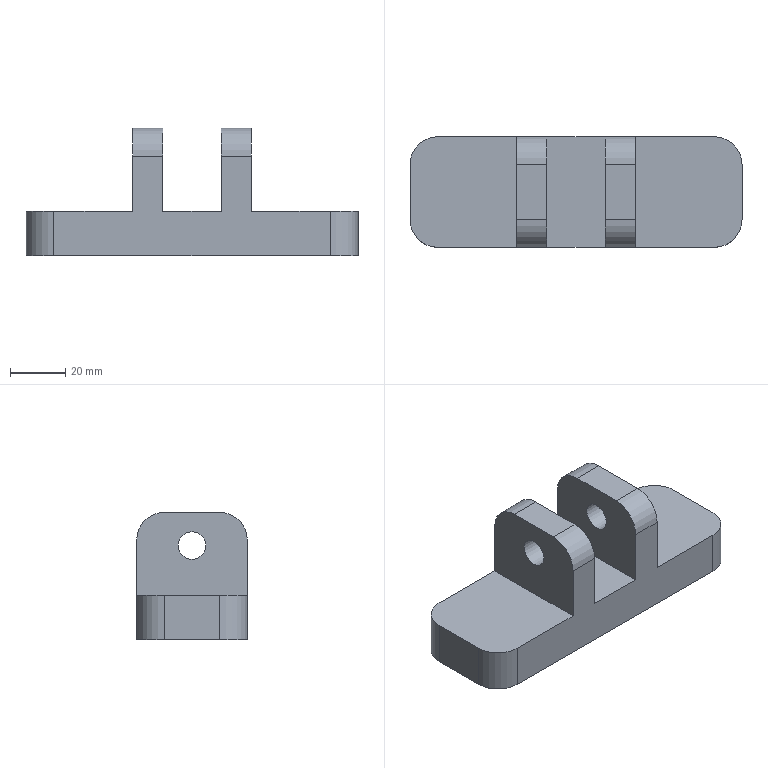Part | NX | 1 solid | 24 faces | box 120 x 40 x 46 mm | volume 99154 mm3 | plane 14 | cylinder 10 | commonest cylinder face diameters 20 x8 10 x2
STEP:
#1=CARTESIAN_POINT('',(81.5,30.,46.));
#2=VERTEX_POINT('',#1);
#3=CARTESIAN_POINT('',(81.5,10.,46.));
#4=VERTEX_POINT('',#3);
#5=CARTESIAN_POINT('',(81.5,20.,46.));
#6=DIRECTION('',(0.,-1.,0.));
#7=VECTOR('',#6,1000.);
#8=LINE('',#5,#7);
#9=EDGE_CURVE('',#2,#4,#8,.T.);
#10=ORIENTED_EDGE('',*,*,#9,.F.);
#11=CARTESIAN_POINT('',(70.5,30.,46.));
#12=VERTEX_POINT('',#11);
#13=CARTESIAN_POINT('',(60.,30.,46.));
#14=DIRECTION('',(1.,0.,0.));
#15=VECTOR('',#14,1000.);
#16=LINE('',#13,#15);
#17=EDGE_CURVE('',#2,#12,#16,.F.);
#18=ORIENTED_EDGE('',*,*,#17,.T.);
#19=CARTESIAN_POINT('',(70.5,10.,46.));
#20=VERTEX_POINT('',#19);
#21=CARTESIAN_POINT('',(70.5,20.,46.));
#22=DIRECTION('',(0.,-1.,0.));
#23=VECTOR('',#22,1000.);
#24=LINE('',#21,#23);
#25=EDGE_CURVE('',#12,#20,#24,.T.);
#26=ORIENTED_EDGE('',*,*,#25,.T.);
#27=CARTESIAN_POINT('',(60.,10.,46.));
#28=DIRECTION('',(-1.,0.,0.));
#29=VECTOR('',#28,1000.);
#30=LINE('',#27,#29);
#31=EDGE_CURVE('',#20,#4,#30,.F.);
#32=ORIENTED_EDGE('',*,*,#31,.T.);
#33=EDGE_LOOP('',(#10,#18,#26,#32));
#34=FACE_BOUND('',#33,.T.);
#35=CARTESIAN_POINT('',(60.,20.,46.));
#36=DIRECTION('',(0.,0.,1.));
#37=DIRECTION('',(1.,0.,0.));
#38=AXIS2_PLACEMENT_3D('',#35,#36,#37);
#39=PLANE('',#38);
#40=ADVANCED_FACE('',(#34),#39,.T.);
#41=CARTESIAN_POINT('',(49.5,10.,46.));
#42=VERTEX_POINT('',#41);
#43=CARTESIAN_POINT('',(49.5,30.,46.));
#44=VERTEX_POINT('',#43);
#45=CARTESIAN_POINT('',(49.5,20.,46.));
#46=DIRECTION('',(0.,1.,0.));
#47=VECTOR('',#46,1000.);
#48=LINE('',#45,#47);
#49=EDGE_CURVE('',#42,#44,#48,.T.);
#50=ORIENTED_EDGE('',*,*,#49,.T.);
#51=CARTESIAN_POINT('',(38.5,30.,46.));
#52=VERTEX_POINT('',#51);
#53=CARTESIAN_POINT('',(60.,30.,46.));
#54=DIRECTION('',(1.,0.,0.));
#55=VECTOR('',#54,1000.);
#56=LINE('',#53,#55);
#57=EDGE_CURVE('',#44,#52,#56,.F.);
#58=ORIENTED_EDGE('',*,*,#57,.T.);
#59=CARTESIAN_POINT('',(38.5,10.,46.));
#60=VERTEX_POINT('',#59);
#61=CARTESIAN_POINT('',(38.5,20.,46.));
#62=DIRECTION('',(0.,1.,0.));
#63=VECTOR('',#62,1000.);
#64=LINE('',#61,#63);
#65=EDGE_CURVE('',#60,#52,#64,.T.);
#66=ORIENTED_EDGE('',*,*,#65,.F.);
#67=CARTESIAN_POINT('',(60.,10.,46.));
#68=DIRECTION('',(-1.,0.,0.));
#69=VECTOR('',#68,1000.);
#70=LINE('',#67,#69);
#71=EDGE_CURVE('',#60,#42,#70,.F.);
#72=ORIENTED_EDGE('',*,*,#71,.T.);
#73=EDGE_LOOP('',(#50,#58,#66,#72));
#74=FACE_BOUND('',#73,.T.);
#75=CARTESIAN_POINT('',(60.,20.,46.));
#76=DIRECTION('',(0.,0.,1.));
#77=DIRECTION('',(1.,0.,0.));
#78=AXIS2_PLACEMENT_3D('',#75,#76,#77);
#79=PLANE('',#78);
#80=ADVANCED_FACE('',(#74),#79,.T.);
#81=CARTESIAN_POINT('',(120.,30.,16.));
#82=VERTEX_POINT('',#81);
#83=CARTESIAN_POINT('',(120.,10.,16.));
#84=VERTEX_POINT('',#83);
#85=CARTESIAN_POINT('',(120.,20.,16.));
#86=DIRECTION('',(0.,-1.,0.));
#87=VECTOR('',#86,1000.);
#88=LINE('',#85,#87);
#89=EDGE_CURVE('',#82,#84,#88,.T.);
#90=ORIENTED_EDGE('',*,*,#89,.F.);
#91=CARTESIAN_POINT('',(110.,40.,16.));
#92=VERTEX_POINT('',#91);
#93=CARTESIAN_POINT('',(110.,30.,16.));
#94=DIRECTION('',(0.,0.,1.));
#95=DIRECTION('',(1.,0.,0.));
#96=AXIS2_PLACEMENT_3D('',#93,#94,#95);
#97=CIRCLE('',#96,10.);
#98=EDGE_CURVE('',#82,#92,#97,.T.);
#99=ORIENTED_EDGE('',*,*,#98,.T.);
#100=CARTESIAN_POINT('',(81.5,40.,16.));
#101=VERTEX_POINT('',#100);
#102=CARTESIAN_POINT('',(60.,40.,16.));
#103=DIRECTION('',(1.,0.,0.));
#104=VECTOR('',#103,1000.);
#105=LINE('',#102,#104);
#106=EDGE_CURVE('',#101,#92,#105,.T.);
#107=ORIENTED_EDGE('',*,*,#106,.F.);
#108=CARTESIAN_POINT('',(81.5,0.,16.));
#109=VERTEX_POINT('',#108);
#110=CARTESIAN_POINT('',(81.5,20.,16.));
#111=DIRECTION('',(0.,1.,0.));
#112=VECTOR('',#111,1000.);
#113=LINE('',#110,#112);
#114=EDGE_CURVE('',#109,#101,#113,.T.);
#115=ORIENTED_EDGE('',*,*,#114,.F.);
#116=CARTESIAN_POINT('',(110.,0.,16.));
#117=VERTEX_POINT('',#116);
#118=CARTESIAN_POINT('',(60.,0.,16.));
#119=DIRECTION('',(-1.,0.,0.));
#120=VECTOR('',#119,1000.);
#121=LINE('',#118,#120);
#122=EDGE_CURVE('',#117,#109,#121,.T.);
#123=ORIENTED_EDGE('',*,*,#122,.F.);
#124=CARTESIAN_POINT('',(110.,10.,16.));
#125=DIRECTION('',(0.,0.,1.));
#126=DIRECTION('',(1.,0.,0.));
#127=AXIS2_PLACEMENT_3D('',#124,#125,#126);
#128=CIRCLE('',#127,10.);
#129=EDGE_CURVE('',#117,#84,#128,.T.);
#130=ORIENTED_EDGE('',*,*,#129,.T.);
#131=EDGE_LOOP('',(#90,#99,#107,#115,#123,#130));
#132=FACE_BOUND('',#131,.T.);
#133=CARTESIAN_POINT('',(60.,20.,16.));
#134=DIRECTION('',(0.,0.,1.));
#135=DIRECTION('',(1.,0.,0.));
#136=AXIS2_PLACEMENT_3D('',#133,#134,#135);
#137=PLANE('',#136);
#138=ADVANCED_FACE('',(#132),#137,.T.);
#139=CARTESIAN_POINT('',(0.,10.,16.));
#140=VERTEX_POINT('',#139);
#141=CARTESIAN_POINT('',(0.,30.,16.));
#142=VERTEX_POINT('',#141);
#143=CARTESIAN_POINT('',(0.,20.,16.));
#144=DIRECTION('',(0.,1.,0.));
#145=VECTOR('',#144,1000.);
#146=LINE('',#143,#145);
#147=EDGE_CURVE('',#140,#142,#146,.T.);
#148=ORIENTED_EDGE('',*,*,#147,.F.);
#149=CARTESIAN_POINT('',(10.,0.,16.));
#150=VERTEX_POINT('',#149);
#151=CARTESIAN_POINT('',(10.,10.,16.));
#152=DIRECTION('',(0.,0.,1.));
#153=DIRECTION('',(1.,0.,0.));
#154=AXIS2_PLACEMENT_3D('',#151,#152,#153);
#155=CIRCLE('',#154,10.);
#156=EDGE_CURVE('',#140,#150,#155,.T.);
#157=ORIENTED_EDGE('',*,*,#156,.T.);
#158=CARTESIAN_POINT('',(38.5,0.,16.));
#159=VERTEX_POINT('',#158);
#160=CARTESIAN_POINT('',(60.,0.,16.));
#161=DIRECTION('',(-1.,0.,0.));
#162=VECTOR('',#161,1000.);
#163=LINE('',#160,#162);
#164=EDGE_CURVE('',#159,#150,#163,.T.);
#165=ORIENTED_EDGE('',*,*,#164,.F.);
#166=CARTESIAN_POINT('',(38.5,40.,16.));
#167=VERTEX_POINT('',#166);
#168=CARTESIAN_POINT('',(38.5,20.,16.));
#169=DIRECTION('',(0.,-1.,0.));
#170=VECTOR('',#169,1000.);
#171=LINE('',#168,#170);
#172=EDGE_CURVE('',#167,#159,#171,.T.);
#173=ORIENTED_EDGE('',*,*,#172,.F.);
#174=CARTESIAN_POINT('',(10.,40.,16.));
#175=VERTEX_POINT('',#174);
#176=CARTESIAN_POINT('',(60.,40.,16.));
#177=DIRECTION('',(1.,0.,0.));
#178=VECTOR('',#177,1000.);
#179=LINE('',#176,#178);
#180=EDGE_CURVE('',#175,#167,#179,.T.);
#181=ORIENTED_EDGE('',*,*,#180,.F.);
#182=CARTESIAN_POINT('',(10.,30.,16.));
#183=DIRECTION('',(0.,0.,1.));
#184=DIRECTION('',(1.,0.,0.));
#185=AXIS2_PLACEMENT_3D('',#182,#183,#184);
#186=CIRCLE('',#185,10.);
#187=EDGE_CURVE('',#175,#142,#186,.T.);
#188=ORIENTED_EDGE('',*,*,#187,.T.);
#189=EDGE_LOOP('',(#148,#157,#165,#173,#181,#188));
#190=FACE_BOUND('',#189,.T.);
#191=CARTESIAN_POINT('',(60.,20.,16.));
#192=DIRECTION('',(0.,0.,1.));
#193=DIRECTION('',(1.,0.,0.));
#194=AXIS2_PLACEMENT_3D('',#191,#192,#193);
#195=PLANE('',#194);
#196=ADVANCED_FACE('',(#190),#195,.T.);
#197=CARTESIAN_POINT('',(49.5,0.,16.));
#198=VERTEX_POINT('',#197);
#199=CARTESIAN_POINT('',(49.5,0.,36.));
#200=VERTEX_POINT('',#199);
#201=CARTESIAN_POINT('',(49.5,0.,16.));
#202=DIRECTION('',(0.,0.,1.));
#203=VECTOR('',#202,1000.);
#204=LINE('',#201,#203);
#205=EDGE_CURVE('',#198,#200,#204,.T.);
#206=ORIENTED_EDGE('',*,*,#205,.T.);
#207=CARTESIAN_POINT('',(38.5,0.,36.));
#208=VERTEX_POINT('',#207);
#209=CARTESIAN_POINT('',(60.,0.,36.));
#210=DIRECTION('',(-1.,0.,0.));
#211=VECTOR('',#210,1000.);
#212=LINE('',#209,#211);
#213=EDGE_CURVE('',#200,#208,#212,.T.);
#214=ORIENTED_EDGE('',*,*,#213,.T.);
#215=CARTESIAN_POINT('',(38.5,0.,16.));
#216=DIRECTION('',(0.,0.,1.));
#217=VECTOR('',#216,1000.);
#218=LINE('',#215,#217);
#219=EDGE_CURVE('',#159,#208,#218,.T.);
#220=ORIENTED_EDGE('',*,*,#219,.F.);
#221=ORIENTED_EDGE('',*,*,#164,.T.);
#222=CARTESIAN_POINT('',(10.,0.,0.));
#223=VERTEX_POINT('',#222);
#224=CARTESIAN_POINT('',(10.,0.,0.));
#225=DIRECTION('',(0.,0.,1.));
#226=VECTOR('',#225,1000.);
#227=LINE('',#224,#226);
#228=EDGE_CURVE('',#150,#223,#227,.F.);
#229=ORIENTED_EDGE('',*,*,#228,.T.);
#230=CARTESIAN_POINT('',(110.,0.,0.));
#231=VERTEX_POINT('',#230);
#232=CARTESIAN_POINT('',(60.,0.,0.));
#233=DIRECTION('',(1.,0.,0.));
#234=VECTOR('',#233,1000.);
#235=LINE('',#232,#234);
#236=EDGE_CURVE('',#223,#231,#235,.T.);
#237=ORIENTED_EDGE('',*,*,#236,.T.);
#238=CARTESIAN_POINT('',(110.,0.,0.));
#239=DIRECTION('',(0.,0.,1.));
#240=VECTOR('',#239,1000.);
#241=LINE('',#238,#240);
#242=EDGE_CURVE('',#231,#117,#241,.T.);
#243=ORIENTED_EDGE('',*,*,#242,.T.);
#244=ORIENTED_EDGE('',*,*,#122,.T.);
#245=CARTESIAN_POINT('',(81.5,0.,36.));
#246=VERTEX_POINT('',#245);
#247=CARTESIAN_POINT('',(81.5,0.,16.));
#248=DIRECTION('',(0.,0.,1.));
#249=VECTOR('',#248,1000.);
#250=LINE('',#247,#249);
#251=EDGE_CURVE('',#109,#246,#250,.T.);
#252=ORIENTED_EDGE('',*,*,#251,.T.);
#253=CARTESIAN_POINT('',(70.5,0.,36.));
#254=VERTEX_POINT('',#253);
#255=CARTESIAN_POINT('',(60.,0.,36.));
#256=DIRECTION('',(-1.,0.,0.));
#257=VECTOR('',#256,1000.);
#258=LINE('',#255,#257);
#259=EDGE_CURVE('',#246,#254,#258,.T.);
#260=ORIENTED_EDGE('',*,*,#259,.T.);
#261=CARTESIAN_POINT('',(70.5,0.,16.));
#262=VERTEX_POINT('',#261);
#263=CARTESIAN_POINT('',(70.5,0.,16.));
#264=DIRECTION('',(0.,0.,1.));
#265=VECTOR('',#264,1000.);
#266=LINE('',#263,#265);
#267=EDGE_CURVE('',#262,#254,#266,.T.);
#268=ORIENTED_EDGE('',*,*,#267,.F.);
#269=CARTESIAN_POINT('',(60.,0.,16.));
#270=DIRECTION('',(1.,0.,0.));
#271=VECTOR('',#270,1000.);
#272=LINE('',#269,#271);
#273=EDGE_CURVE('',#198,#262,#272,.T.);
#274=ORIENTED_EDGE('',*,*,#273,.F.);
#275=EDGE_LOOP('',(#206,#214,#220,#221,#229,#237,#243,#244,#252,#260,#268,#274));
#276=FACE_BOUND('',#275,.T.);
#277=CARTESIAN_POINT('',(60.,0.,0.));
#278=DIRECTION('',(0.,-1.,0.));
#279=DIRECTION('',(0.,0.,-1.));
#280=AXIS2_PLACEMENT_3D('',#277,#278,#279);
#281=PLANE('',#280);
#282=ADVANCED_FACE('',(#276),#281,.T.);
#283=CARTESIAN_POINT('',(0.,30.,0.));
#284=VERTEX_POINT('',#283);
#285=CARTESIAN_POINT('',(0.,10.,0.));
#286=VERTEX_POINT('',#285);
#287=CARTESIAN_POINT('',(0.,20.,0.));
#288=DIRECTION('',(0.,-1.,0.));
#289=VECTOR('',#288,1000.);
#290=LINE('',#287,#289);
#291=EDGE_CURVE('',#284,#286,#290,.T.);
#292=ORIENTED_EDGE('',*,*,#291,.T.);
#293=CARTESIAN_POINT('',(0.,10.,0.));
#294=DIRECTION('',(0.,0.,1.));
#295=VECTOR('',#294,1000.);
#296=LINE('',#293,#295);
#297=EDGE_CURVE('',#286,#140,#296,.T.);
#298=ORIENTED_EDGE('',*,*,#297,.T.);
#299=ORIENTED_EDGE('',*,*,#147,.T.);
#300=CARTESIAN_POINT('',(0.,30.,0.));
#301=DIRECTION('',(0.,0.,1.));
#302=VECTOR('',#301,1000.);
#303=LINE('',#300,#302);
#304=EDGE_CURVE('',#142,#284,#303,.F.);
#305=ORIENTED_EDGE('',*,*,#304,.T.);
#306=EDGE_LOOP('',(#292,#298,#299,#305));
#307=FACE_BOUND('',#306,.T.);
#308=CARTESIAN_POINT('',(0.,20.,0.));
#309=DIRECTION('',(-1.,0.,0.));
#310=DIRECTION('',(0.,0.,1.));
#311=AXIS2_PLACEMENT_3D('',#308,#309,#310);
#312=PLANE('',#311);
#313=ADVANCED_FACE('',(#307),#312,.T.);
#314=CARTESIAN_POINT('',(70.5,40.,16.));
#315=VERTEX_POINT('',#314);
#316=CARTESIAN_POINT('',(70.5,40.,36.));
#317=VERTEX_POINT('',#316);
#318=CARTESIAN_POINT('',(70.5,40.,16.));
#319=DIRECTION('',(0.,0.,1.));
#320=VECTOR('',#319,1000.);
#321=LINE('',#318,#320);
#322=EDGE_CURVE('',#315,#317,#321,.T.);
#323=ORIENTED_EDGE('',*,*,#322,.T.);
#324=CARTESIAN_POINT('',(81.5,40.,36.));
#325=VERTEX_POINT('',#324);
#326=CARTESIAN_POINT('',(60.,40.,36.));
#327=DIRECTION('',(1.,0.,0.));
#328=VECTOR('',#327,1000.);
#329=LINE('',#326,#328);
#330=EDGE_CURVE('',#317,#325,#329,.T.);
#331=ORIENTED_EDGE('',*,*,#330,.T.);
#332=CARTESIAN_POINT('',(81.5,40.,16.));
#333=DIRECTION('',(0.,0.,1.));
#334=VECTOR('',#333,1000.);
#335=LINE('',#332,#334);
#336=EDGE_CURVE('',#101,#325,#335,.T.);
#337=ORIENTED_EDGE('',*,*,#336,.F.);
#338=ORIENTED_EDGE('',*,*,#106,.T.);
#339=CARTESIAN_POINT('',(110.,40.,0.));
#340=VERTEX_POINT('',#339);
#341=CARTESIAN_POINT('',(110.,40.,0.));
#342=DIRECTION('',(0.,0.,1.));
#343=VECTOR('',#342,1000.);
#344=LINE('',#341,#343);
#345=EDGE_CURVE('',#92,#340,#344,.F.);
#346=ORIENTED_EDGE('',*,*,#345,.T.);
#347=CARTESIAN_POINT('',(10.,40.,0.));
#348=VERTEX_POINT('',#347);
#349=CARTESIAN_POINT('',(60.,40.,0.));
#350=DIRECTION('',(-1.,0.,0.));
#351=VECTOR('',#350,1000.);
#352=LINE('',#349,#351);
#353=EDGE_CURVE('',#340,#348,#352,.T.);
#354=ORIENTED_EDGE('',*,*,#353,.T.);
#355=CARTESIAN_POINT('',(10.,40.,0.));
#356=DIRECTION('',(0.,0.,1.));
#357=VECTOR('',#356,1000.);
#358=LINE('',#355,#357);
#359=EDGE_CURVE('',#348,#175,#358,.T.);
#360=ORIENTED_EDGE('',*,*,#359,.T.);
#361=ORIENTED_EDGE('',*,*,#180,.T.);
#362=CARTESIAN_POINT('',(38.5,40.,36.));
#363=VERTEX_POINT('',#362);
#364=CARTESIAN_POINT('',(38.5,40.,16.));
#365=DIRECTION('',(0.,0.,1.));
#366=VECTOR('',#365,1000.);
#367=LINE('',#364,#366);
#368=EDGE_CURVE('',#167,#363,#367,.T.);
#369=ORIENTED_EDGE('',*,*,#368,.T.);
#370=CARTESIAN_POINT('',(49.5,40.,36.));
#371=VERTEX_POINT('',#370);
#372=CARTESIAN_POINT('',(60.,40.,36.));
#373=DIRECTION('',(1.,0.,0.));
#374=VECTOR('',#373,1000.);
#375=LINE('',#372,#374);
#376=EDGE_CURVE('',#363,#371,#375,.T.);
#377=ORIENTED_EDGE('',*,*,#376,.T.);
#378=CARTESIAN_POINT('',(49.5,40.,16.));
#379=VERTEX_POINT('',#378);
#380=CARTESIAN_POINT('',(49.5,40.,16.));
#381=DIRECTION('',(0.,0.,1.));
#382=VECTOR('',#381,1000.);
#383=LINE('',#380,#382);
#384=EDGE_CURVE('',#379,#371,#383,.T.);
#385=ORIENTED_EDGE('',*,*,#384,.F.);
#386=CARTESIAN_POINT('',(60.,40.,16.));
#387=DIRECTION('',(-1.,0.,0.));
#388=VECTOR('',#387,1000.);
#389=LINE('',#386,#388);
#390=EDGE_CURVE('',#315,#379,#389,.T.);
#391=ORIENTED_EDGE('',*,*,#390,.F.);
#392=EDGE_LOOP('',(#323,#331,#337,#338,#346,#354,#360,#361,#369,#377,#385,#391));
#393=FACE_BOUND('',#392,.T.);
#394=CARTESIAN_POINT('',(60.,40.,0.));
#395=DIRECTION('',(0.,1.,0.));
#396=DIRECTION('',(0.,0.,1.));
#397=AXIS2_PLACEMENT_3D('',#394,#395,#396);
#398=PLANE('',#397);
#399=ADVANCED_FACE('',(#393),#398,.T.);
#400=ORIENTED_EDGE('',*,*,#236,.F.);
#401=CARTESIAN_POINT('',(10.,10.,0.));
#402=DIRECTION('',(0.,0.,-1.));
#403=DIRECTION('',(-1.,0.,0.));
#404=AXIS2_PLACEMENT_3D('',#401,#402,#403);
#405=CIRCLE('',#404,10.);
#406=EDGE_CURVE('',#223,#286,#405,.T.);
#407=ORIENTED_EDGE('',*,*,#406,.T.);
#408=ORIENTED_EDGE('',*,*,#291,.F.);
#409=CARTESIAN_POINT('',(10.,30.,0.));
#410=DIRECTION('',(0.,0.,-1.));
#411=DIRECTION('',(-1.,0.,0.));
#412=AXIS2_PLACEMENT_3D('',#409,#410,#411);
#413=CIRCLE('',#412,10.);
#414=EDGE_CURVE('',#284,#348,#413,.T.);
#415=ORIENTED_EDGE('',*,*,#414,.T.);
#416=ORIENTED_EDGE('',*,*,#353,.F.);
#417=CARTESIAN_POINT('',(120.,30.,0.));
#418=VERTEX_POINT('',#417);
#419=CARTESIAN_POINT('',(110.,30.,0.));
#420=DIRECTION('',(0.,0.,-1.));
#421=DIRECTION('',(-1.,0.,0.));
#422=AXIS2_PLACEMENT_3D('',#419,#420,#421);
#423=CIRCLE('',#422,10.);
#424=EDGE_CURVE('',#340,#418,#423,.T.);
#425=ORIENTED_EDGE('',*,*,#424,.T.);
#426=CARTESIAN_POINT('',(120.,10.,0.));
#427=VERTEX_POINT('',#426);
#428=CARTESIAN_POINT('',(120.,20.,0.));
#429=DIRECTION('',(0.,1.,0.));
#430=VECTOR('',#429,1000.);
#431=LINE('',#428,#430);
#432=EDGE_CURVE('',#427,#418,#431,.T.);
#433=ORIENTED_EDGE('',*,*,#432,.F.);
#434=CARTESIAN_POINT('',(110.,10.,0.));
#435=DIRECTION('',(0.,0.,-1.));
#436=DIRECTION('',(-1.,0.,0.));
#437=AXIS2_PLACEMENT_3D('',#434,#435,#436);
#438=CIRCLE('',#437,10.);
#439=EDGE_CURVE('',#427,#231,#438,.T.);
#440=ORIENTED_EDGE('',*,*,#439,.T.);
#441=EDGE_LOOP('',(#400,#407,#408,#415,#416,#425,#433,#440));
#442=FACE_BOUND('',#441,.T.);
#443=CARTESIAN_POINT('',(60.,20.,0.));
#444=DIRECTION('',(0.,0.,-1.));
#445=DIRECTION('',(-1.,0.,0.));
#446=AXIS2_PLACEMENT_3D('',#443,#444,#445);
#447=PLANE('',#446);
#448=ADVANCED_FACE('',(#442),#447,.T.);
#449=ORIENTED_EDGE('',*,*,#432,.T.);
#450=CARTESIAN_POINT('',(120.,30.,0.));
#451=DIRECTION('',(0.,0.,1.));
#452=VECTOR('',#451,1000.);
#453=LINE('',#450,#452);
#454=EDGE_CURVE('',#418,#82,#453,.T.);
#455=ORIENTED_EDGE('',*,*,#454,.T.);
#456=ORIENTED_EDGE('',*,*,#89,.T.);
#457=CARTESIAN_POINT('',(120.,10.,0.));
#458=DIRECTION('',(0.,0.,1.));
#459=VECTOR('',#458,1000.);
#460=LINE('',#457,#459);
#461=EDGE_CURVE('',#84,#427,#460,.F.);
#462=ORIENTED_EDGE('',*,*,#461,.T.);
#463=EDGE_LOOP('',(#449,#455,#456,#462));
#464=FACE_BOUND('',#463,.T.);
#465=CARTESIAN_POINT('',(120.,20.,0.));
#466=DIRECTION('',(1.,0.,0.));
#467=DIRECTION('',(0.,0.,-1.));
#468=AXIS2_PLACEMENT_3D('',#465,#466,#467);
#469=PLANE('',#468);
#470=ADVANCED_FACE('',(#464),#469,.T.);
#471=CARTESIAN_POINT('',(38.5,20.,39.));
#472=VERTEX_POINT('',#471);
#473=CARTESIAN_POINT('',(38.5,20.,34.));
#474=DIRECTION('',(-1.,0.,0.));
#475=DIRECTION('',(0.,0.,1.));
#476=AXIS2_PLACEMENT_3D('',#473,#474,#475);
#477=CIRCLE('',#476,5.);
#478=EDGE_CURVE('',#472,#472,#477,.T.);
#479=ORIENTED_EDGE('',*,*,#478,.F.);
#480=EDGE_LOOP('',(#479));
#481=FACE_BOUND('',#480,.T.);
#482=ORIENTED_EDGE('',*,*,#65,.T.);
#483=CARTESIAN_POINT('',(38.5,30.,36.));
#484=DIRECTION('',(-1.,0.,0.));
#485=DIRECTION('',(0.,0.,1.));
#486=AXIS2_PLACEMENT_3D('',#483,#484,#485);
#487=CIRCLE('',#486,10.);
#488=EDGE_CURVE('',#52,#363,#487,.T.);
#489=ORIENTED_EDGE('',*,*,#488,.T.);
#490=ORIENTED_EDGE('',*,*,#368,.F.);
#491=ORIENTED_EDGE('',*,*,#172,.T.);
#492=ORIENTED_EDGE('',*,*,#219,.T.);
#493=CARTESIAN_POINT('',(38.5,10.,36.));
#494=DIRECTION('',(-1.,0.,0.));
#495=DIRECTION('',(0.,0.,1.));
#496=AXIS2_PLACEMENT_3D('',#493,#494,#495);
#497=CIRCLE('',#496,10.);
#498=EDGE_CURVE('',#208,#60,#497,.T.);
#499=ORIENTED_EDGE('',*,*,#498,.T.);
#500=EDGE_LOOP('',(#482,#489,#490,#491,#492,#499));
#501=FACE_BOUND('',#500,.T.);
#502=CARTESIAN_POINT('',(38.5,20.,16.));
#503=DIRECTION('',(-1.,0.,0.));
#504=DIRECTION('',(0.,0.,1.));
#505=AXIS2_PLACEMENT_3D('',#502,#503,#504);
#506=PLANE('',#505);
#507=ADVANCED_FACE('',(#481,#501),#506,.T.);
#508=CARTESIAN_POINT('',(81.5,20.,29.));
#509=VERTEX_POINT('',#508);
#510=CARTESIAN_POINT('',(81.5,20.,34.));
#511=DIRECTION('',(1.,0.,0.));
#512=DIRECTION('',(0.,0.,-1.));
#513=AXIS2_PLACEMENT_3D('',#510,#511,#512);
#514=CIRCLE('',#513,5.);
#515=EDGE_CURVE('',#509,#509,#514,.T.);
#516=ORIENTED_EDGE('',*,*,#515,.F.);
#517=EDGE_LOOP('',(#516));
#518=FACE_BOUND('',#517,.T.);
#519=ORIENTED_EDGE('',*,*,#336,.T.);
#520=CARTESIAN_POINT('',(81.5,30.,36.));
#521=DIRECTION('',(1.,0.,0.));
#522=DIRECTION('',(0.,0.,-1.));
#523=AXIS2_PLACEMENT_3D('',#520,#521,#522);
#524=CIRCLE('',#523,10.);
#525=EDGE_CURVE('',#325,#2,#524,.T.);
#526=ORIENTED_EDGE('',*,*,#525,.T.);
#527=ORIENTED_EDGE('',*,*,#9,.T.);
#528=CARTESIAN_POINT('',(81.5,10.,36.));
#529=DIRECTION('',(1.,0.,0.));
#530=DIRECTION('',(0.,0.,-1.));
#531=AXIS2_PLACEMENT_3D('',#528,#529,#530);
#532=CIRCLE('',#531,10.);
#533=EDGE_CURVE('',#4,#246,#532,.T.);
#534=ORIENTED_EDGE('',*,*,#533,.T.);
#535=ORIENTED_EDGE('',*,*,#251,.F.);
#536=ORIENTED_EDGE('',*,*,#114,.T.);
#537=EDGE_LOOP('',(#519,#526,#527,#534,#535,#536));
#538=FACE_BOUND('',#537,.T.);
#539=CARTESIAN_POINT('',(81.5,20.,16.));
#540=DIRECTION('',(1.,0.,0.));
#541=DIRECTION('',(0.,0.,-1.));
#542=AXIS2_PLACEMENT_3D('',#539,#540,#541);
#543=PLANE('',#542);
#544=ADVANCED_FACE('',(#518,#538),#543,.T.);
#545=CARTESIAN_POINT('',(49.5,20.,39.));
#546=VERTEX_POINT('',#545);
#547=CARTESIAN_POINT('',(49.5,20.,34.));
#548=DIRECTION('',(-1.,0.,0.));
#549=DIRECTION('',(0.,0.,1.));
#550=AXIS2_PLACEMENT_3D('',#547,#548,#549);
#551=CIRCLE('',#550,5.);
#552=EDGE_CURVE('',#546,#546,#551,.T.);
#553=ORIENTED_EDGE('',*,*,#552,.T.);
#554=EDGE_LOOP('',(#553));
#555=FACE_BOUND('',#554,.T.);
#556=ORIENTED_EDGE('',*,*,#384,.T.);
#557=CARTESIAN_POINT('',(49.5,30.,36.));
#558=DIRECTION('',(-1.,0.,0.));
#559=DIRECTION('',(0.,0.,1.));
#560=AXIS2_PLACEMENT_3D('',#557,#558,#559);
#561=CIRCLE('',#560,10.);
#562=EDGE_CURVE('',#371,#44,#561,.F.);
#563=ORIENTED_EDGE('',*,*,#562,.T.);
#564=ORIENTED_EDGE('',*,*,#49,.F.);
#565=CARTESIAN_POINT('',(49.5,10.,36.));
#566=DIRECTION('',(-1.,0.,0.));
#567=DIRECTION('',(0.,0.,1.));
#568=AXIS2_PLACEMENT_3D('',#565,#566,#567);
#569=CIRCLE('',#568,10.);
#570=EDGE_CURVE('',#42,#200,#569,.F.);
#571=ORIENTED_EDGE('',*,*,#570,.T.);
#572=ORIENTED_EDGE('',*,*,#205,.F.);
#573=CARTESIAN_POINT('',(49.5,20.,16.));
#574=DIRECTION('',(0.,-1.,0.));
#575=VECTOR('',#574,1000.);
#576=LINE('',#573,#575);
#577=EDGE_CURVE('',#198,#379,#576,.F.);
#578=ORIENTED_EDGE('',*,*,#577,.T.);
#579=EDGE_LOOP('',(#556,#563,#564,#571,#572,#578));
#580=FACE_BOUND('',#579,.T.);
#581=CARTESIAN_POINT('',(49.5,20.,16.));
#582=DIRECTION('',(-1.,0.,0.));
#583=DIRECTION('',(0.,0.,1.));
#584=AXIS2_PLACEMENT_3D('',#581,#582,#583);
#585=PLANE('',#584);
#586=ADVANCED_FACE('',(#555,#580),#585,.F.);
#587=CARTESIAN_POINT('',(70.5,20.,16.));
#588=DIRECTION('',(0.,1.,0.));
#589=VECTOR('',#588,1000.);
#590=LINE('',#587,#589);
#591=EDGE_CURVE('',#315,#262,#590,.F.);
#592=ORIENTED_EDGE('',*,*,#591,.F.);
#593=ORIENTED_EDGE('',*,*,#390,.T.);
#594=ORIENTED_EDGE('',*,*,#577,.F.);
#595=ORIENTED_EDGE('',*,*,#273,.T.);
#596=EDGE_LOOP('',(#592,#593,#594,#595));
#597=FACE_BOUND('',#596,.T.);
#598=CARTESIAN_POINT('',(60.,20.,16.));
#599=DIRECTION('',(0.,0.,-1.));
#600=DIRECTION('',(-1.,0.,0.));
#601=AXIS2_PLACEMENT_3D('',#598,#599,#600);
#602=PLANE('',#601);
#603=ADVANCED_FACE('',(#597),#602,.F.);
#604=CARTESIAN_POINT('',(70.5,20.,29.));
#605=VERTEX_POINT('',#604);
#606=CARTESIAN_POINT('',(70.5,20.,34.));
#607=DIRECTION('',(1.,0.,0.));
#608=DIRECTION('',(0.,0.,-1.));
#609=AXIS2_PLACEMENT_3D('',#606,#607,#608);
#610=CIRCLE('',#609,5.);
#611=EDGE_CURVE('',#605,#605,#610,.T.);
#612=ORIENTED_EDGE('',*,*,#611,.T.);
#613=EDGE_LOOP('',(#612));
#614=FACE_BOUND('',#613,.T.);
#615=ORIENTED_EDGE('',*,*,#25,.F.);
#616=CARTESIAN_POINT('',(70.5,30.,36.));
#617=DIRECTION('',(1.,0.,0.));
#618=DIRECTION('',(0.,0.,-1.));
#619=AXIS2_PLACEMENT_3D('',#616,#617,#618);
#620=CIRCLE('',#619,10.);
#621=EDGE_CURVE('',#12,#317,#620,.F.);
#622=ORIENTED_EDGE('',*,*,#621,.T.);
#623=ORIENTED_EDGE('',*,*,#322,.F.);
#624=ORIENTED_EDGE('',*,*,#591,.T.);
#625=ORIENTED_EDGE('',*,*,#267,.T.);
#626=CARTESIAN_POINT('',(70.5,10.,36.));
#627=DIRECTION('',(1.,0.,0.));
#628=DIRECTION('',(0.,0.,-1.));
#629=AXIS2_PLACEMENT_3D('',#626,#627,#628);
#630=CIRCLE('',#629,10.);
#631=EDGE_CURVE('',#254,#20,#630,.F.);
#632=ORIENTED_EDGE('',*,*,#631,.T.);
#633=EDGE_LOOP('',(#615,#622,#623,#624,#625,#632));
#634=FACE_BOUND('',#633,.T.);
#635=CARTESIAN_POINT('',(70.5,20.,16.));
#636=DIRECTION('',(1.,0.,0.));
#637=DIRECTION('',(0.,0.,-1.));
#638=AXIS2_PLACEMENT_3D('',#635,#636,#637);
#639=PLANE('',#638);
#640=ADVANCED_FACE('',(#614,#634),#639,.F.);
#641=ORIENTED_EDGE('',*,*,#406,.F.);
#642=ORIENTED_EDGE('',*,*,#228,.F.);
#643=ORIENTED_EDGE('',*,*,#156,.F.);
#644=ORIENTED_EDGE('',*,*,#297,.F.);
#645=EDGE_LOOP('',(#641,#642,#643,#644));
#646=FACE_BOUND('',#645,.T.);
#647=CARTESIAN_POINT('',(10.,10.,0.));
#648=DIRECTION('',(0.,0.,1.));
#649=DIRECTION('',(1.,0.,0.));
#650=AXIS2_PLACEMENT_3D('',#647,#648,#649);
#651=CYLINDRICAL_SURFACE('',#650,10.);
#652=ADVANCED_FACE('',(#646),#651,.T.);
#653=ORIENTED_EDGE('',*,*,#414,.F.);
#654=ORIENTED_EDGE('',*,*,#304,.F.);
#655=ORIENTED_EDGE('',*,*,#187,.F.);
#656=ORIENTED_EDGE('',*,*,#359,.F.);
#657=EDGE_LOOP('',(#653,#654,#655,#656));
#658=FACE_BOUND('',#657,.T.);
#659=CARTESIAN_POINT('',(10.,30.,0.));
#660=DIRECTION('',(0.,0.,1.));
#661=DIRECTION('',(1.,0.,0.));
#662=AXIS2_PLACEMENT_3D('',#659,#660,#661);
#663=CYLINDRICAL_SURFACE('',#662,10.);
#664=ADVANCED_FACE('',(#658),#663,.T.);
#665=ORIENTED_EDGE('',*,*,#424,.F.);
#666=ORIENTED_EDGE('',*,*,#345,.F.);
#667=ORIENTED_EDGE('',*,*,#98,.F.);
#668=ORIENTED_EDGE('',*,*,#454,.F.);
#669=EDGE_LOOP('',(#665,#666,#667,#668));
#670=FACE_BOUND('',#669,.T.);
#671=CARTESIAN_POINT('',(110.,30.,0.));
#672=DIRECTION('',(0.,0.,1.));
#673=DIRECTION('',(1.,0.,0.));
#674=AXIS2_PLACEMENT_3D('',#671,#672,#673);
#675=CYLINDRICAL_SURFACE('',#674,10.);
#676=ADVANCED_FACE('',(#670),#675,.T.);
#677=ORIENTED_EDGE('',*,*,#439,.F.);
#678=ORIENTED_EDGE('',*,*,#461,.F.);
#679=ORIENTED_EDGE('',*,*,#129,.F.);
#680=ORIENTED_EDGE('',*,*,#242,.F.);
#681=EDGE_LOOP('',(#677,#678,#679,#680));
#682=FACE_BOUND('',#681,.T.);
#683=CARTESIAN_POINT('',(110.,10.,0.));
#684=DIRECTION('',(0.,0.,1.));
#685=DIRECTION('',(1.,0.,0.));
#686=AXIS2_PLACEMENT_3D('',#683,#684,#685);
#687=CYLINDRICAL_SURFACE('',#686,10.);
#688=ADVANCED_FACE('',(#682),#687,.T.);
#689=ORIENTED_EDGE('',*,*,#621,.F.);
#690=ORIENTED_EDGE('',*,*,#17,.F.);
#691=ORIENTED_EDGE('',*,*,#525,.F.);
#692=ORIENTED_EDGE('',*,*,#330,.F.);
#693=EDGE_LOOP('',(#689,#690,#691,#692));
#694=FACE_BOUND('',#693,.T.);
#695=CARTESIAN_POINT('',(60.,30.,36.));
#696=DIRECTION('',(1.,0.,0.));
#697=DIRECTION('',(0.,0.,-1.));
#698=AXIS2_PLACEMENT_3D('',#695,#696,#697);
#699=CYLINDRICAL_SURFACE('',#698,10.);
#700=ADVANCED_FACE('',(#694),#699,.T.);
#701=ORIENTED_EDGE('',*,*,#488,.F.);
#702=ORIENTED_EDGE('',*,*,#57,.F.);
#703=ORIENTED_EDGE('',*,*,#562,.F.);
#704=ORIENTED_EDGE('',*,*,#376,.F.);
#705=EDGE_LOOP('',(#701,#702,#703,#704));
#706=FACE_BOUND('',#705,.T.);
#707=CARTESIAN_POINT('',(60.,30.,36.));
#708=DIRECTION('',(1.,0.,0.));
#709=DIRECTION('',(0.,0.,-1.));
#710=AXIS2_PLACEMENT_3D('',#707,#708,#709);
#711=CYLINDRICAL_SURFACE('',#710,10.);
#712=ADVANCED_FACE('',(#706),#711,.T.);
#713=ORIENTED_EDGE('',*,*,#570,.F.);
#714=ORIENTED_EDGE('',*,*,#71,.F.);
#715=ORIENTED_EDGE('',*,*,#498,.F.);
#716=ORIENTED_EDGE('',*,*,#213,.F.);
#717=EDGE_LOOP('',(#713,#714,#715,#716));
#718=FACE_BOUND('',#717,.T.);
#719=CARTESIAN_POINT('',(60.,10.,36.));
#720=DIRECTION('',(-1.,0.,0.));
#721=DIRECTION('',(0.,0.,1.));
#722=AXIS2_PLACEMENT_3D('',#719,#720,#721);
#723=CYLINDRICAL_SURFACE('',#722,10.);
#724=ADVANCED_FACE('',(#718),#723,.T.);
#725=ORIENTED_EDGE('',*,*,#533,.F.);
#726=ORIENTED_EDGE('',*,*,#31,.F.);
#727=ORIENTED_EDGE('',*,*,#631,.F.);
#728=ORIENTED_EDGE('',*,*,#259,.F.);
#729=EDGE_LOOP('',(#725,#726,#727,#728));
#730=FACE_BOUND('',#729,.T.);
#731=CARTESIAN_POINT('',(60.,10.,36.));
#732=DIRECTION('',(-1.,0.,0.));
#733=DIRECTION('',(0.,0.,1.));
#734=AXIS2_PLACEMENT_3D('',#731,#732,#733);
#735=CYLINDRICAL_SURFACE('',#734,10.);
#736=ADVANCED_FACE('',(#730),#735,.T.);
#737=ORIENTED_EDGE('',*,*,#515,.T.);
#738=EDGE_LOOP('',(#737));
#739=FACE_BOUND('',#738,.T.);
#740=ORIENTED_EDGE('',*,*,#611,.F.);
#741=EDGE_LOOP('',(#740));
#742=FACE_BOUND('',#741,.T.);
#743=CARTESIAN_POINT('',(0.,20.,34.));
#744=DIRECTION('',(1.,0.,0.));
#745=DIRECTION('',(0.,0.,-1.));
#746=AXIS2_PLACEMENT_3D('',#743,#744,#745);
#747=CYLINDRICAL_SURFACE('',#746,5.);
#748=ADVANCED_FACE('',(#739,#742),#747,.F.);
#749=ORIENTED_EDGE('',*,*,#478,.T.);
#750=EDGE_LOOP('',(#749));
#751=FACE_BOUND('',#750,.T.);
#752=ORIENTED_EDGE('',*,*,#552,.F.);
#753=EDGE_LOOP('',(#752));
#754=FACE_BOUND('',#753,.T.);
#755=CARTESIAN_POINT('',(0.,20.,34.));
#756=DIRECTION('',(1.,0.,0.));
#757=DIRECTION('',(0.,0.,-1.));
#758=AXIS2_PLACEMENT_3D('',#755,#756,#757);
#759=CYLINDRICAL_SURFACE('',#758,5.);
#760=ADVANCED_FACE('',(#751,#754),#759,.F.);
#761=CLOSED_SHELL('',(#40,#80,#138,#196,#282,#313,#399,#448,#470,#507,#544,#586,#603,#640,#652,#664,#676,#688,#700,#712,#724,#736,#748,#760));
#762=MANIFOLD_SOLID_BREP('',#761);
#763=(LENGTH_UNIT()NAMED_UNIT(*)SI_UNIT(.MILLI.,.METRE.));
#764=UNCERTAINTY_MEASURE_WITH_UNIT(LENGTH_MEASURE(0.00001),#763,'','');
#765=(NAMED_UNIT(*)PLANE_ANGLE_UNIT()SI_UNIT($,.RADIAN.));
#766=(NAMED_UNIT(*)SI_UNIT($,.STERADIAN.)SOLID_ANGLE_UNIT());
#767=(GEOMETRIC_REPRESENTATION_CONTEXT(3)GLOBAL_UNCERTAINTY_ASSIGNED_CONTEXT((#764))GLOBAL_UNIT_ASSIGNED_CONTEXT((#763,#765,#766))REPRESENTATION_CONTEXT('',''));
#768=ADVANCED_BREP_SHAPE_REPRESENTATION('',(#762),#767);